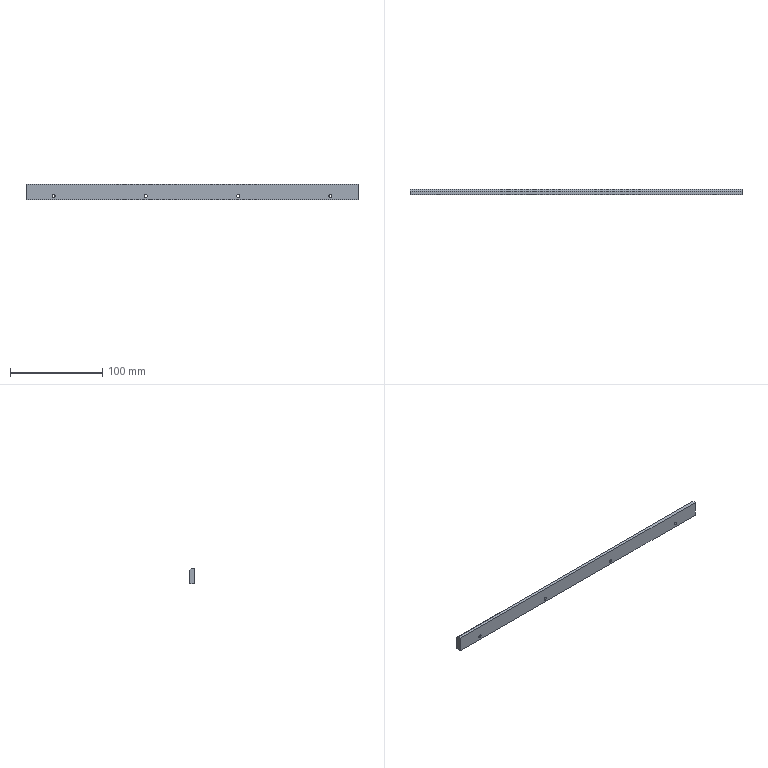Part | STEP file | PN_0029 | 1 solid | 15 faces | box 360 x 5.4 x 16.8 mm | volume 31743 mm3 | cylinder 8 | plane 7 | commonest cylinder face diameters 3.4 x8
STEP:
#1=CARTESIAN_POINT('',(0.,0.,0.));
#2=DIRECTION('',(0.,0.,1.));
#3=DIRECTION('',(1.,0.,0.));
#4=AXIS2_PLACEMENT_3D('',#1,#2,#3);
#5=CARTESIAN_POINT('',(-150.,0.,-2.7));
#6=VERTEX_POINT('',#5);
#7=CARTESIAN_POINT('',(-150.,5.4,-2.7));
#8=VERTEX_POINT('',#7);
#9=CARTESIAN_POINT('',(-150.,5.4,-2.7));
#10=DIRECTION('',(0.,1.,0.));
#11=VECTOR('',#10,1.);
#12=LINE('',#9,#11);
#13=CARTESIAN_POINT('',(-150.,5.4,-4.4));
#14=DIRECTION('',(0.,1.,0.));
#15=DIRECTION('',(0.,0.,1.));
#16=AXIS2_PLACEMENT_3D('',#13,#14,#15);
#17=CYLINDRICAL_SURFACE('',#16,1.7);
#18=CARTESIAN_POINT('',(6.283,0.));
#19=DIRECTION('',(0.,1.));
#20=VECTOR('',#19,1.);
#21=LINE('',#18,#20);
#22=(GEOMETRIC_REPRESENTATION_CONTEXT(2)PARAMETRIC_REPRESENTATION_CONTEXT()REPRESENTATION_CONTEXT('',''));
#23=DEFINITIONAL_REPRESENTATION('',(#21),#22);
#24=PCURVE('',#17,#23);
#25=CARTESIAN_POINT('',(-150.,5.4,-4.4));
#26=DIRECTION('',(0.,1.,0.));
#27=DIRECTION('',(0.,0.,1.));
#28=AXIS2_PLACEMENT_3D('',#25,#26,#27);
#29=CYLINDRICAL_SURFACE('',#28,1.7);
#30=CARTESIAN_POINT('',(0.,0.));
#31=DIRECTION('',(0.,1.));
#32=VECTOR('',#31,1.);
#33=LINE('',#30,#32);
#34=(GEOMETRIC_REPRESENTATION_CONTEXT(2)PARAMETRIC_REPRESENTATION_CONTEXT()REPRESENTATION_CONTEXT('',''));
#35=DEFINITIONAL_REPRESENTATION('',(#33),#34);
#36=PCURVE('',#29,#35);
#37=SURFACE_CURVE('',#12,(#24,#36),.PCURVE_S1.);
#38=EDGE_CURVE('',#6,#8,#37,.T.);
#39=ORIENTED_EDGE('',*,*,#38,.T.);
#40=CARTESIAN_POINT('',(-150.,5.4,-6.1));
#41=VERTEX_POINT('',#40);
#42=CARTESIAN_POINT('',(-150.,5.4,-4.4));
#43=DIRECTION('',(0.,1.,0.));
#44=DIRECTION('',(0.,0.,1.));
#45=AXIS2_PLACEMENT_3D('',#42,#43,#44);
#46=CIRCLE('',#45,1.7);
#47=CARTESIAN_POINT('',(0.,0.));
#48=DIRECTION('',(1.,0.));
#49=VECTOR('',#48,1.);
#50=LINE('',#47,#49);
#51=(GEOMETRIC_REPRESENTATION_CONTEXT(2)PARAMETRIC_REPRESENTATION_CONTEXT()REPRESENTATION_CONTEXT('',''));
#52=DEFINITIONAL_REPRESENTATION('',(#50),#51);
#53=PCURVE('',#17,#52);
#54=CARTESIAN_POINT('',(0.,5.4,0.));
#55=DIRECTION('',(0.,1.,0.));
#56=DIRECTION('',(0.,0.,1.));
#57=AXIS2_PLACEMENT_3D('',#54,#55,#56);
#58=PLANE('',#57);
#59=CARTESIAN_POINT('',(-4.4,-150.));
#60=DIRECTION('',(1.,0.));
#61=AXIS2_PLACEMENT_2D('',#59,#60);
#62=CIRCLE('',#61,1.7);
#63=(GEOMETRIC_REPRESENTATION_CONTEXT(2)PARAMETRIC_REPRESENTATION_CONTEXT()REPRESENTATION_CONTEXT('',''));
#64=DEFINITIONAL_REPRESENTATION('',(#62),#63);
#65=PCURVE('',#58,#64);
#66=SURFACE_CURVE('',#46,(#53,#65),.PCURVE_S1.);
#67=EDGE_CURVE('',#41,#8,#66,.T.);
#68=ORIENTED_EDGE('',*,*,#67,.F.);
#69=CARTESIAN_POINT('',(-150.,0.,-6.1));
#70=VERTEX_POINT('',#69);
#71=CARTESIAN_POINT('',(-150.,5.4,-6.1));
#72=DIRECTION('',(0.,1.,0.));
#73=VECTOR('',#72,1.);
#74=LINE('',#71,#73);
#75=CARTESIAN_POINT('',(3.142,0.));
#76=DIRECTION('',(0.,1.));
#77=VECTOR('',#76,1.);
#78=LINE('',#75,#77);
#79=(GEOMETRIC_REPRESENTATION_CONTEXT(2)PARAMETRIC_REPRESENTATION_CONTEXT()REPRESENTATION_CONTEXT('',''));
#80=DEFINITIONAL_REPRESENTATION('',(#78),#79);
#81=PCURVE('',#17,#80);
#82=CARTESIAN_POINT('',(3.142,0.));
#83=DIRECTION('',(0.,1.));
#84=VECTOR('',#83,1.);
#85=LINE('',#82,#84);
#86=(GEOMETRIC_REPRESENTATION_CONTEXT(2)PARAMETRIC_REPRESENTATION_CONTEXT()REPRESENTATION_CONTEXT('',''));
#87=DEFINITIONAL_REPRESENTATION('',(#85),#86);
#88=PCURVE('',#29,#87);
#89=SURFACE_CURVE('',#74,(#81,#88),.PCURVE_S1.);
#90=EDGE_CURVE('',#70,#41,#89,.T.);
#91=ORIENTED_EDGE('',*,*,#90,.F.);
#92=CARTESIAN_POINT('',(-150.,0.,-4.4));
#93=DIRECTION('',(0.,1.,0.));
#94=DIRECTION('',(0.,0.,1.));
#95=AXIS2_PLACEMENT_3D('',#92,#93,#94);
#96=CIRCLE('',#95,1.7);
#97=CARTESIAN_POINT('',(0.,-5.4));
#98=DIRECTION('',(1.,0.));
#99=VECTOR('',#98,1.);
#100=LINE('',#97,#99);
#101=(GEOMETRIC_REPRESENTATION_CONTEXT(2)PARAMETRIC_REPRESENTATION_CONTEXT()REPRESENTATION_CONTEXT('',''));
#102=DEFINITIONAL_REPRESENTATION('',(#100),#101);
#103=PCURVE('',#17,#102);
#104=CARTESIAN_POINT('',(0.,0.,0.));
#105=DIRECTION('',(0.,1.,0.));
#106=DIRECTION('',(0.,0.,1.));
#107=AXIS2_PLACEMENT_3D('',#104,#105,#106);
#108=PLANE('',#107);
#109=CARTESIAN_POINT('',(-4.4,-150.));
#110=DIRECTION('',(1.,0.));
#111=AXIS2_PLACEMENT_2D('',#109,#110);
#112=CIRCLE('',#111,1.7);
#113=(GEOMETRIC_REPRESENTATION_CONTEXT(2)PARAMETRIC_REPRESENTATION_CONTEXT()REPRESENTATION_CONTEXT('',''));
#114=DEFINITIONAL_REPRESENTATION('',(#112),#113);
#115=PCURVE('',#108,#114);
#116=SURFACE_CURVE('',#96,(#103,#115),.PCURVE_S1.);
#117=EDGE_CURVE('',#70,#6,#116,.T.);
#118=ORIENTED_EDGE('',*,*,#117,.T.);
#119=EDGE_LOOP('',(#39,#68,#91,#118));
#120=FACE_BOUND('',#119,.F.);
#121=ADVANCED_FACE('',(#120),#17,.F.);
#122=CARTESIAN_POINT('',(-50.,0.,-2.7));
#123=VERTEX_POINT('',#122);
#124=CARTESIAN_POINT('',(-50.,5.4,-2.7));
#125=VERTEX_POINT('',#124);
#126=CARTESIAN_POINT('',(-50.,5.4,-2.7));
#127=DIRECTION('',(0.,1.,0.));
#128=VECTOR('',#127,1.);
#129=LINE('',#126,#128);
#130=CARTESIAN_POINT('',(-50.,5.4,-4.4));
#131=DIRECTION('',(0.,1.,0.));
#132=DIRECTION('',(0.,0.,1.));
#133=AXIS2_PLACEMENT_3D('',#130,#131,#132);
#134=CYLINDRICAL_SURFACE('',#133,1.7);
#135=CARTESIAN_POINT('',(6.283,0.));
#136=DIRECTION('',(0.,1.));
#137=VECTOR('',#136,1.);
#138=LINE('',#135,#137);
#139=(GEOMETRIC_REPRESENTATION_CONTEXT(2)PARAMETRIC_REPRESENTATION_CONTEXT()REPRESENTATION_CONTEXT('',''));
#140=DEFINITIONAL_REPRESENTATION('',(#138),#139);
#141=PCURVE('',#134,#140);
#142=CARTESIAN_POINT('',(-50.,5.4,-4.4));
#143=DIRECTION('',(0.,1.,0.));
#144=DIRECTION('',(0.,0.,1.));
#145=AXIS2_PLACEMENT_3D('',#142,#143,#144);
#146=CYLINDRICAL_SURFACE('',#145,1.7);
#147=CARTESIAN_POINT('',(0.,0.));
#148=DIRECTION('',(0.,1.));
#149=VECTOR('',#148,1.);
#150=LINE('',#147,#149);
#151=(GEOMETRIC_REPRESENTATION_CONTEXT(2)PARAMETRIC_REPRESENTATION_CONTEXT()REPRESENTATION_CONTEXT('',''));
#152=DEFINITIONAL_REPRESENTATION('',(#150),#151);
#153=PCURVE('',#146,#152);
#154=SURFACE_CURVE('',#129,(#141,#153),.PCURVE_S1.);
#155=EDGE_CURVE('',#123,#125,#154,.T.);
#156=ORIENTED_EDGE('',*,*,#155,.T.);
#157=CARTESIAN_POINT('',(-50.,5.4,-6.1));
#158=VERTEX_POINT('',#157);
#159=CARTESIAN_POINT('',(-50.,5.4,-4.4));
#160=DIRECTION('',(0.,1.,0.));
#161=DIRECTION('',(0.,0.,1.));
#162=AXIS2_PLACEMENT_3D('',#159,#160,#161);
#163=CIRCLE('',#162,1.7);
#164=CARTESIAN_POINT('',(0.,0.));
#165=DIRECTION('',(1.,0.));
#166=VECTOR('',#165,1.);
#167=LINE('',#164,#166);
#168=(GEOMETRIC_REPRESENTATION_CONTEXT(2)PARAMETRIC_REPRESENTATION_CONTEXT()REPRESENTATION_CONTEXT('',''));
#169=DEFINITIONAL_REPRESENTATION('',(#167),#168);
#170=PCURVE('',#134,#169);
#171=CARTESIAN_POINT('',(-4.4,-50.));
#172=DIRECTION('',(1.,0.));
#173=AXIS2_PLACEMENT_2D('',#171,#172);
#174=CIRCLE('',#173,1.7);
#175=(GEOMETRIC_REPRESENTATION_CONTEXT(2)PARAMETRIC_REPRESENTATION_CONTEXT()REPRESENTATION_CONTEXT('',''));
#176=DEFINITIONAL_REPRESENTATION('',(#174),#175);
#177=PCURVE('',#58,#176);
#178=SURFACE_CURVE('',#163,(#170,#177),.PCURVE_S1.);
#179=EDGE_CURVE('',#158,#125,#178,.T.);
#180=ORIENTED_EDGE('',*,*,#179,.F.);
#181=CARTESIAN_POINT('',(-50.,0.,-6.1));
#182=VERTEX_POINT('',#181);
#183=CARTESIAN_POINT('',(-50.,5.4,-6.1));
#184=DIRECTION('',(0.,1.,0.));
#185=VECTOR('',#184,1.);
#186=LINE('',#183,#185);
#187=CARTESIAN_POINT('',(3.142,0.));
#188=DIRECTION('',(0.,1.));
#189=VECTOR('',#188,1.);
#190=LINE('',#187,#189);
#191=(GEOMETRIC_REPRESENTATION_CONTEXT(2)PARAMETRIC_REPRESENTATION_CONTEXT()REPRESENTATION_CONTEXT('',''));
#192=DEFINITIONAL_REPRESENTATION('',(#190),#191);
#193=PCURVE('',#134,#192);
#194=CARTESIAN_POINT('',(3.142,0.));
#195=DIRECTION('',(0.,1.));
#196=VECTOR('',#195,1.);
#197=LINE('',#194,#196);
#198=(GEOMETRIC_REPRESENTATION_CONTEXT(2)PARAMETRIC_REPRESENTATION_CONTEXT()REPRESENTATION_CONTEXT('',''));
#199=DEFINITIONAL_REPRESENTATION('',(#197),#198);
#200=PCURVE('',#146,#199);
#201=SURFACE_CURVE('',#186,(#193,#200),.PCURVE_S1.);
#202=EDGE_CURVE('',#182,#158,#201,.T.);
#203=ORIENTED_EDGE('',*,*,#202,.F.);
#204=CARTESIAN_POINT('',(-50.,0.,-4.4));
#205=DIRECTION('',(0.,1.,0.));
#206=DIRECTION('',(0.,0.,1.));
#207=AXIS2_PLACEMENT_3D('',#204,#205,#206);
#208=CIRCLE('',#207,1.7);
#209=CARTESIAN_POINT('',(0.,-5.4));
#210=DIRECTION('',(1.,0.));
#211=VECTOR('',#210,1.);
#212=LINE('',#209,#211);
#213=(GEOMETRIC_REPRESENTATION_CONTEXT(2)PARAMETRIC_REPRESENTATION_CONTEXT()REPRESENTATION_CONTEXT('',''));
#214=DEFINITIONAL_REPRESENTATION('',(#212),#213);
#215=PCURVE('',#134,#214);
#216=CARTESIAN_POINT('',(-4.4,-50.));
#217=DIRECTION('',(1.,0.));
#218=AXIS2_PLACEMENT_2D('',#216,#217);
#219=CIRCLE('',#218,1.7);
#220=(GEOMETRIC_REPRESENTATION_CONTEXT(2)PARAMETRIC_REPRESENTATION_CONTEXT()REPRESENTATION_CONTEXT('',''));
#221=DEFINITIONAL_REPRESENTATION('',(#219),#220);
#222=PCURVE('',#108,#221);
#223=SURFACE_CURVE('',#208,(#215,#222),.PCURVE_S1.);
#224=EDGE_CURVE('',#182,#123,#223,.T.);
#225=ORIENTED_EDGE('',*,*,#224,.T.);
#226=EDGE_LOOP('',(#156,#180,#203,#225));
#227=FACE_BOUND('',#226,.F.);
#228=ADVANCED_FACE('',(#227),#134,.F.);
#229=CARTESIAN_POINT('',(50.,0.,-2.7));
#230=VERTEX_POINT('',#229);
#231=CARTESIAN_POINT('',(50.,5.4,-2.7));
#232=VERTEX_POINT('',#231);
#233=CARTESIAN_POINT('',(50.,5.4,-2.7));
#234=DIRECTION('',(0.,1.,0.));
#235=VECTOR('',#234,1.);
#236=LINE('',#233,#235);
#237=CARTESIAN_POINT('',(50.,5.4,-4.4));
#238=DIRECTION('',(0.,1.,0.));
#239=DIRECTION('',(0.,0.,1.));
#240=AXIS2_PLACEMENT_3D('',#237,#238,#239);
#241=CYLINDRICAL_SURFACE('',#240,1.7);
#242=CARTESIAN_POINT('',(6.283,0.));
#243=DIRECTION('',(0.,1.));
#244=VECTOR('',#243,1.);
#245=LINE('',#242,#244);
#246=(GEOMETRIC_REPRESENTATION_CONTEXT(2)PARAMETRIC_REPRESENTATION_CONTEXT()REPRESENTATION_CONTEXT('',''));
#247=DEFINITIONAL_REPRESENTATION('',(#245),#246);
#248=PCURVE('',#241,#247);
#249=CARTESIAN_POINT('',(50.,5.4,-4.4));
#250=DIRECTION('',(0.,1.,0.));
#251=DIRECTION('',(0.,0.,1.));
#252=AXIS2_PLACEMENT_3D('',#249,#250,#251);
#253=CYLINDRICAL_SURFACE('',#252,1.7);
#254=CARTESIAN_POINT('',(0.,0.));
#255=DIRECTION('',(0.,1.));
#256=VECTOR('',#255,1.);
#257=LINE('',#254,#256);
#258=(GEOMETRIC_REPRESENTATION_CONTEXT(2)PARAMETRIC_REPRESENTATION_CONTEXT()REPRESENTATION_CONTEXT('',''));
#259=DEFINITIONAL_REPRESENTATION('',(#257),#258);
#260=PCURVE('',#253,#259);
#261=SURFACE_CURVE('',#236,(#248,#260),.PCURVE_S1.);
#262=EDGE_CURVE('',#230,#232,#261,.T.);
#263=ORIENTED_EDGE('',*,*,#262,.T.);
#264=CARTESIAN_POINT('',(50.,5.4,-6.1));
#265=VERTEX_POINT('',#264);
#266=CARTESIAN_POINT('',(50.,5.4,-4.4));
#267=DIRECTION('',(0.,1.,0.));
#268=DIRECTION('',(0.,0.,1.));
#269=AXIS2_PLACEMENT_3D('',#266,#267,#268);
#270=CIRCLE('',#269,1.7);
#271=CARTESIAN_POINT('',(0.,0.));
#272=DIRECTION('',(1.,0.));
#273=VECTOR('',#272,1.);
#274=LINE('',#271,#273);
#275=(GEOMETRIC_REPRESENTATION_CONTEXT(2)PARAMETRIC_REPRESENTATION_CONTEXT()REPRESENTATION_CONTEXT('',''));
#276=DEFINITIONAL_REPRESENTATION('',(#274),#275);
#277=PCURVE('',#241,#276);
#278=CARTESIAN_POINT('',(-4.4,50.));
#279=DIRECTION('',(1.,0.));
#280=AXIS2_PLACEMENT_2D('',#278,#279);
#281=CIRCLE('',#280,1.7);
#282=(GEOMETRIC_REPRESENTATION_CONTEXT(2)PARAMETRIC_REPRESENTATION_CONTEXT()REPRESENTATION_CONTEXT('',''));
#283=DEFINITIONAL_REPRESENTATION('',(#281),#282);
#284=PCURVE('',#58,#283);
#285=SURFACE_CURVE('',#270,(#277,#284),.PCURVE_S1.);
#286=EDGE_CURVE('',#265,#232,#285,.T.);
#287=ORIENTED_EDGE('',*,*,#286,.F.);
#288=CARTESIAN_POINT('',(50.,0.,-6.1));
#289=VERTEX_POINT('',#288);
#290=CARTESIAN_POINT('',(50.,5.4,-6.1));
#291=DIRECTION('',(0.,1.,0.));
#292=VECTOR('',#291,1.);
#293=LINE('',#290,#292);
#294=CARTESIAN_POINT('',(3.142,0.));
#295=DIRECTION('',(0.,1.));
#296=VECTOR('',#295,1.);
#297=LINE('',#294,#296);
#298=(GEOMETRIC_REPRESENTATION_CONTEXT(2)PARAMETRIC_REPRESENTATION_CONTEXT()REPRESENTATION_CONTEXT('',''));
#299=DEFINITIONAL_REPRESENTATION('',(#297),#298);
#300=PCURVE('',#241,#299);
#301=CARTESIAN_POINT('',(3.142,0.));
#302=DIRECTION('',(0.,1.));
#303=VECTOR('',#302,1.);
#304=LINE('',#301,#303);
#305=(GEOMETRIC_REPRESENTATION_CONTEXT(2)PARAMETRIC_REPRESENTATION_CONTEXT()REPRESENTATION_CONTEXT('',''));
#306=DEFINITIONAL_REPRESENTATION('',(#304),#305);
#307=PCURVE('',#253,#306);
#308=SURFACE_CURVE('',#293,(#300,#307),.PCURVE_S1.);
#309=EDGE_CURVE('',#289,#265,#308,.T.);
#310=ORIENTED_EDGE('',*,*,#309,.F.);
#311=CARTESIAN_POINT('',(50.,0.,-4.4));
#312=DIRECTION('',(0.,1.,0.));
#313=DIRECTION('',(0.,0.,1.));
#314=AXIS2_PLACEMENT_3D('',#311,#312,#313);
#315=CIRCLE('',#314,1.7);
#316=CARTESIAN_POINT('',(0.,-5.4));
#317=DIRECTION('',(1.,0.));
#318=VECTOR('',#317,1.);
#319=LINE('',#316,#318);
#320=(GEOMETRIC_REPRESENTATION_CONTEXT(2)PARAMETRIC_REPRESENTATION_CONTEXT()REPRESENTATION_CONTEXT('',''));
#321=DEFINITIONAL_REPRESENTATION('',(#319),#320);
#322=PCURVE('',#241,#321);
#323=CARTESIAN_POINT('',(-4.4,50.));
#324=DIRECTION('',(1.,0.));
#325=AXIS2_PLACEMENT_2D('',#323,#324);
#326=CIRCLE('',#325,1.7);
#327=(GEOMETRIC_REPRESENTATION_CONTEXT(2)PARAMETRIC_REPRESENTATION_CONTEXT()REPRESENTATION_CONTEXT('',''));
#328=DEFINITIONAL_REPRESENTATION('',(#326),#327);
#329=PCURVE('',#108,#328);
#330=SURFACE_CURVE('',#315,(#322,#329),.PCURVE_S1.);
#331=EDGE_CURVE('',#289,#230,#330,.T.);
#332=ORIENTED_EDGE('',*,*,#331,.T.);
#333=EDGE_LOOP('',(#263,#287,#310,#332));
#334=FACE_BOUND('',#333,.F.);
#335=ADVANCED_FACE('',(#334),#241,.F.);
#336=CARTESIAN_POINT('',(150.,0.,-2.7));
#337=VERTEX_POINT('',#336);
#338=CARTESIAN_POINT('',(150.,5.4,-2.7));
#339=VERTEX_POINT('',#338);
#340=CARTESIAN_POINT('',(150.,5.4,-2.7));
#341=DIRECTION('',(0.,1.,0.));
#342=VECTOR('',#341,1.);
#343=LINE('',#340,#342);
#344=CARTESIAN_POINT('',(150.,5.4,-4.4));
#345=DIRECTION('',(0.,1.,0.));
#346=DIRECTION('',(0.,0.,1.));
#347=AXIS2_PLACEMENT_3D('',#344,#345,#346);
#348=CYLINDRICAL_SURFACE('',#347,1.7);
#349=CARTESIAN_POINT('',(6.283,0.));
#350=DIRECTION('',(0.,1.));
#351=VECTOR('',#350,1.);
#352=LINE('',#349,#351);
#353=(GEOMETRIC_REPRESENTATION_CONTEXT(2)PARAMETRIC_REPRESENTATION_CONTEXT()REPRESENTATION_CONTEXT('',''));
#354=DEFINITIONAL_REPRESENTATION('',(#352),#353);
#355=PCURVE('',#348,#354);
#356=CARTESIAN_POINT('',(150.,5.4,-4.4));
#357=DIRECTION('',(0.,1.,0.));
#358=DIRECTION('',(0.,0.,1.));
#359=AXIS2_PLACEMENT_3D('',#356,#357,#358);
#360=CYLINDRICAL_SURFACE('',#359,1.7);
#361=CARTESIAN_POINT('',(0.,0.));
#362=DIRECTION('',(0.,1.));
#363=VECTOR('',#362,1.);
#364=LINE('',#361,#363);
#365=(GEOMETRIC_REPRESENTATION_CONTEXT(2)PARAMETRIC_REPRESENTATION_CONTEXT()REPRESENTATION_CONTEXT('',''));
#366=DEFINITIONAL_REPRESENTATION('',(#364),#365);
#367=PCURVE('',#360,#366);
#368=SURFACE_CURVE('',#343,(#355,#367),.PCURVE_S1.);
#369=EDGE_CURVE('',#337,#339,#368,.T.);
#370=ORIENTED_EDGE('',*,*,#369,.T.);
#371=CARTESIAN_POINT('',(150.,5.4,-6.1));
#372=VERTEX_POINT('',#371);
#373=CARTESIAN_POINT('',(150.,5.4,-4.4));
#374=DIRECTION('',(0.,1.,0.));
#375=DIRECTION('',(0.,0.,1.));
#376=AXIS2_PLACEMENT_3D('',#373,#374,#375);
#377=CIRCLE('',#376,1.7);
#378=CARTESIAN_POINT('',(0.,0.));
#379=DIRECTION('',(1.,0.));
#380=VECTOR('',#379,1.);
#381=LINE('',#378,#380);
#382=(GEOMETRIC_REPRESENTATION_CONTEXT(2)PARAMETRIC_REPRESENTATION_CONTEXT()REPRESENTATION_CONTEXT('',''));
#383=DEFINITIONAL_REPRESENTATION('',(#381),#382);
#384=PCURVE('',#348,#383);
#385=CARTESIAN_POINT('',(-4.4,150.));
#386=DIRECTION('',(1.,0.));
#387=AXIS2_PLACEMENT_2D('',#385,#386);
#388=CIRCLE('',#387,1.7);
#389=(GEOMETRIC_REPRESENTATION_CONTEXT(2)PARAMETRIC_REPRESENTATION_CONTEXT()REPRESENTATION_CONTEXT('',''));
#390=DEFINITIONAL_REPRESENTATION('',(#388),#389);
#391=PCURVE('',#58,#390);
#392=SURFACE_CURVE('',#377,(#384,#391),.PCURVE_S1.);
#393=EDGE_CURVE('',#372,#339,#392,.T.);
#394=ORIENTED_EDGE('',*,*,#393,.F.);
#395=CARTESIAN_POINT('',(150.,0.,-6.1));
#396=VERTEX_POINT('',#395);
#397=CARTESIAN_POINT('',(150.,5.4,-6.1));
#398=DIRECTION('',(0.,1.,0.));
#399=VECTOR('',#398,1.);
#400=LINE('',#397,#399);
#401=CARTESIAN_POINT('',(3.142,0.));
#402=DIRECTION('',(0.,1.));
#403=VECTOR('',#402,1.);
#404=LINE('',#401,#403);
#405=(GEOMETRIC_REPRESENTATION_CONTEXT(2)PARAMETRIC_REPRESENTATION_CONTEXT()REPRESENTATION_CONTEXT('',''));
#406=DEFINITIONAL_REPRESENTATION('',(#404),#405);
#407=PCURVE('',#348,#406);
#408=CARTESIAN_POINT('',(3.142,0.));
#409=DIRECTION('',(0.,1.));
#410=VECTOR('',#409,1.);
#411=LINE('',#408,#410);
#412=(GEOMETRIC_REPRESENTATION_CONTEXT(2)PARAMETRIC_REPRESENTATION_CONTEXT()REPRESENTATION_CONTEXT('',''));
#413=DEFINITIONAL_REPRESENTATION('',(#411),#412);
#414=PCURVE('',#360,#413);
#415=SURFACE_CURVE('',#400,(#407,#414),.PCURVE_S1.);
#416=EDGE_CURVE('',#396,#372,#415,.T.);
#417=ORIENTED_EDGE('',*,*,#416,.F.);
#418=CARTESIAN_POINT('',(150.,0.,-4.4));
#419=DIRECTION('',(0.,1.,0.));
#420=DIRECTION('',(0.,0.,1.));
#421=AXIS2_PLACEMENT_3D('',#418,#419,#420);
#422=CIRCLE('',#421,1.7);
#423=CARTESIAN_POINT('',(0.,-5.4));
#424=DIRECTION('',(1.,0.));
#425=VECTOR('',#424,1.);
#426=LINE('',#423,#425);
#427=(GEOMETRIC_REPRESENTATION_CONTEXT(2)PARAMETRIC_REPRESENTATION_CONTEXT()REPRESENTATION_CONTEXT('',''));
#428=DEFINITIONAL_REPRESENTATION('',(#426),#427);
#429=PCURVE('',#348,#428);
#430=CARTESIAN_POINT('',(-4.4,150.));
#431=DIRECTION('',(1.,0.));
#432=AXIS2_PLACEMENT_2D('',#430,#431);
#433=CIRCLE('',#432,1.7);
#434=(GEOMETRIC_REPRESENTATION_CONTEXT(2)PARAMETRIC_REPRESENTATION_CONTEXT()REPRESENTATION_CONTEXT('',''));
#435=DEFINITIONAL_REPRESENTATION('',(#433),#434);
#436=PCURVE('',#108,#435);
#437=SURFACE_CURVE('',#422,(#429,#436),.PCURVE_S1.);
#438=EDGE_CURVE('',#396,#337,#437,.T.);
#439=ORIENTED_EDGE('',*,*,#438,.T.);
#440=EDGE_LOOP('',(#370,#394,#417,#439));
#441=FACE_BOUND('',#440,.F.);
#442=ADVANCED_FACE('',(#441),#348,.F.);
#443=CARTESIAN_POINT('',(180.,5.4,6.4));
#444=VERTEX_POINT('',#443);
#445=CARTESIAN_POINT('',(180.,5.4,-8.4));
#446=VERTEX_POINT('',#445);
#447=CARTESIAN_POINT('',(180.,5.4,-8.4));
#448=DIRECTION('',(0.,0.,-1.));
#449=VECTOR('',#448,1.);
#450=LINE('',#447,#449);
#451=CARTESIAN_POINT('',(180.,5.4,-8.4));
#452=DIRECTION('',(-1.,0.,0.));
#453=DIRECTION('',(0.,0.,1.));
#454=AXIS2_PLACEMENT_3D('',#451,#452,#453);
#455=PLANE('',#454);
#456=CARTESIAN_POINT('',(0.,0.));
#457=DIRECTION('',(-1.,0.));
#458=VECTOR('',#457,1.);
#459=LINE('',#456,#458);
#460=(GEOMETRIC_REPRESENTATION_CONTEXT(2)PARAMETRIC_REPRESENTATION_CONTEXT()REPRESENTATION_CONTEXT('',''));
#461=DEFINITIONAL_REPRESENTATION('',(#459),#460);
#462=PCURVE('',#455,#461);
#463=CARTESIAN_POINT('',(-8.4,180.));
#464=DIRECTION('',(-1.,0.));
#465=VECTOR('',#464,1.);
#466=LINE('',#463,#465);
#467=(GEOMETRIC_REPRESENTATION_CONTEXT(2)PARAMETRIC_REPRESENTATION_CONTEXT()REPRESENTATION_CONTEXT('',''));
#468=DEFINITIONAL_REPRESENTATION('',(#466),#467);
#469=PCURVE('',#58,#468);
#470=SURFACE_CURVE('',#450,(#462,#469),.PCURVE_S1.);
#471=EDGE_CURVE('',#444,#446,#470,.T.);
#472=ORIENTED_EDGE('',*,*,#471,.F.);
#473=CARTESIAN_POINT('',(180.,3.4,8.4));
#474=VERTEX_POINT('',#473);
#475=CARTESIAN_POINT('',(180.,3.4,8.4));
#476=DIRECTION('',(0.,-0.7071,0.7071));
#477=VECTOR('',#476,1.);
#478=LINE('',#475,#477);
#479=CARTESIAN_POINT('',(16.8,-2.));
#480=DIRECTION('',(0.7071,-0.7071));
#481=VECTOR('',#480,1.);
#482=LINE('',#479,#481);
#483=(GEOMETRIC_REPRESENTATION_CONTEXT(2)PARAMETRIC_REPRESENTATION_CONTEXT()REPRESENTATION_CONTEXT('',''));
#484=DEFINITIONAL_REPRESENTATION('',(#482),#483);
#485=PCURVE('',#455,#484);
#486=CARTESIAN_POINT('',(180.,3.4,8.4));
#487=DIRECTION('',(0.,-0.7071,-0.7071));
#488=DIRECTION('',(0.,0.7071,-0.7071));
#489=AXIS2_PLACEMENT_3D('',#486,#487,#488);
#490=PLANE('',#489);
#491=CARTESIAN_POINT('',(0.,0.));
#492=DIRECTION('',(-1.,0.));
#493=VECTOR('',#492,1.);
#494=LINE('',#491,#493);
#495=(GEOMETRIC_REPRESENTATION_CONTEXT(2)PARAMETRIC_REPRESENTATION_CONTEXT()REPRESENTATION_CONTEXT('',''));
#496=DEFINITIONAL_REPRESENTATION('',(#494),#495);
#497=PCURVE('',#490,#496);
#498=SURFACE_CURVE('',#478,(#485,#497),.PCURVE_S1.);
#499=EDGE_CURVE('',#444,#474,#498,.T.);
#500=ORIENTED_EDGE('',*,*,#499,.T.);
#501=CARTESIAN_POINT('',(180.,0.,8.4));
#502=VERTEX_POINT('',#501);
#503=CARTESIAN_POINT('',(180.,5.4,8.4));
#504=DIRECTION('',(0.,-1.,0.));
#505=VECTOR('',#504,1.);
#506=LINE('',#503,#505);
#507=CARTESIAN_POINT('',(16.8,0.));
#508=DIRECTION('',(0.,-1.));
#509=VECTOR('',#508,1.);
#510=LINE('',#507,#509);
#511=(GEOMETRIC_REPRESENTATION_CONTEXT(2)PARAMETRIC_REPRESENTATION_CONTEXT()REPRESENTATION_CONTEXT('',''));
#512=DEFINITIONAL_REPRESENTATION('',(#510),#511);
#513=PCURVE('',#455,#512);
#514=CARTESIAN_POINT('',(-180.,5.4,8.4));
#515=DIRECTION('',(0.,0.,-1.));
#516=DIRECTION('',(-1.,0.,0.));
#517=AXIS2_PLACEMENT_3D('',#514,#515,#516);
#518=PLANE('',#517);
#519=CARTESIAN_POINT('',(-360.,0.));
#520=DIRECTION('',(0.,-1.));
#521=VECTOR('',#520,1.);
#522=LINE('',#519,#521);
#523=(GEOMETRIC_REPRESENTATION_CONTEXT(2)PARAMETRIC_REPRESENTATION_CONTEXT()REPRESENTATION_CONTEXT('',''));
#524=DEFINITIONAL_REPRESENTATION('',(#522),#523);
#525=PCURVE('',#518,#524);
#526=SURFACE_CURVE('',#506,(#513,#525),.PCURVE_S1.);
#527=EDGE_CURVE('',#474,#502,#526,.T.);
#528=ORIENTED_EDGE('',*,*,#527,.T.);
#529=CARTESIAN_POINT('',(180.,0.,-8.4));
#530=VERTEX_POINT('',#529);
#531=CARTESIAN_POINT('',(180.,0.,-8.4));
#532=DIRECTION('',(0.,0.,-1.));
#533=VECTOR('',#532,1.);
#534=LINE('',#531,#533);
#535=CARTESIAN_POINT('',(0.,-5.4));
#536=DIRECTION('',(-1.,0.));
#537=VECTOR('',#536,1.);
#538=LINE('',#535,#537);
#539=(GEOMETRIC_REPRESENTATION_CONTEXT(2)PARAMETRIC_REPRESENTATION_CONTEXT()REPRESENTATION_CONTEXT('',''));
#540=DEFINITIONAL_REPRESENTATION('',(#538),#539);
#541=PCURVE('',#455,#540);
#542=CARTESIAN_POINT('',(-8.4,180.));
#543=DIRECTION('',(-1.,0.));
#544=VECTOR('',#543,1.);
#545=LINE('',#542,#544);
#546=(GEOMETRIC_REPRESENTATION_CONTEXT(2)PARAMETRIC_REPRESENTATION_CONTEXT()REPRESENTATION_CONTEXT('',''));
#547=DEFINITIONAL_REPRESENTATION('',(#545),#546);
#548=PCURVE('',#108,#547);
#549=SURFACE_CURVE('',#534,(#541,#548),.PCURVE_S1.);
#550=EDGE_CURVE('',#502,#530,#549,.T.);
#551=ORIENTED_EDGE('',*,*,#550,.T.);
#552=CARTESIAN_POINT('',(180.,5.4,-8.4));
#553=DIRECTION('',(0.,-1.,0.));
#554=VECTOR('',#553,1.);
#555=LINE('',#552,#554);
#556=CARTESIAN_POINT('',(0.,0.));
#557=DIRECTION('',(0.,-1.));
#558=VECTOR('',#557,1.);
#559=LINE('',#556,#558);
#560=(GEOMETRIC_REPRESENTATION_CONTEXT(2)PARAMETRIC_REPRESENTATION_CONTEXT()REPRESENTATION_CONTEXT('',''));
#561=DEFINITIONAL_REPRESENTATION('',(#559),#560);
#562=PCURVE('',#455,#561);
#563=CARTESIAN_POINT('',(-180.,5.4,-8.4));
#564=DIRECTION('',(0.,0.,1.));
#565=DIRECTION('',(1.,0.,0.));
#566=AXIS2_PLACEMENT_3D('',#563,#564,#565);
#567=PLANE('',#566);
#568=CARTESIAN_POINT('',(360.,0.));
#569=DIRECTION('',(0.,-1.));
#570=VECTOR('',#569,1.);
#571=LINE('',#568,#570);
#572=(GEOMETRIC_REPRESENTATION_CONTEXT(2)PARAMETRIC_REPRESENTATION_CONTEXT()REPRESENTATION_CONTEXT('',''));
#573=DEFINITIONAL_REPRESENTATION('',(#571),#572);
#574=PCURVE('',#567,#573);
#575=SURFACE_CURVE('',#555,(#562,#574),.PCURVE_S1.);
#576=EDGE_CURVE('',#446,#530,#575,.T.);
#577=ORIENTED_EDGE('',*,*,#576,.F.);
#578=EDGE_LOOP('',(#472,#500,#528,#551,#577));
#579=FACE_BOUND('',#578,.T.);
#580=ADVANCED_FACE('',(#579),#455,.F.);
#581=CARTESIAN_POINT('',(-180.,0.,-8.4));
#582=VERTEX_POINT('',#581);
#583=CARTESIAN_POINT('',(-180.,0.,-8.4));
#584=DIRECTION('',(-1.,0.,0.));
#585=VECTOR('',#584,1.);
#586=LINE('',#583,#585);
#587=CARTESIAN_POINT('',(0.,-5.4));
#588=DIRECTION('',(-1.,0.));
#589=VECTOR('',#588,1.);
#590=LINE('',#587,#589);
#591=(GEOMETRIC_REPRESENTATION_CONTEXT(2)PARAMETRIC_REPRESENTATION_CONTEXT()REPRESENTATION_CONTEXT('',''));
#592=DEFINITIONAL_REPRESENTATION('',(#590),#591);
#593=PCURVE('',#567,#592);
#594=CARTESIAN_POINT('',(-8.4,-180.));
#595=DIRECTION('',(0.,-1.));
#596=VECTOR('',#595,1.);
#597=LINE('',#594,#596);
#598=(GEOMETRIC_REPRESENTATION_CONTEXT(2)PARAMETRIC_REPRESENTATION_CONTEXT()REPRESENTATION_CONTEXT('',''));
#599=DEFINITIONAL_REPRESENTATION('',(#597),#598);
#600=PCURVE('',#108,#599);
#601=SURFACE_CURVE('',#586,(#593,#600),.PCURVE_S1.);
#602=EDGE_CURVE('',#530,#582,#601,.T.);
#603=ORIENTED_EDGE('',*,*,#602,.T.);
#604=CARTESIAN_POINT('',(-180.,5.4,-8.4));
#605=VERTEX_POINT('',#604);
#606=CARTESIAN_POINT('',(-180.,5.4,-8.4));
#607=DIRECTION('',(0.,-1.,0.));
#608=VECTOR('',#607,1.);
#609=LINE('',#606,#608);
#610=CARTESIAN_POINT('',(0.,0.));
#611=DIRECTION('',(0.,-1.));
#612=VECTOR('',#611,1.);
#613=LINE('',#610,#612);
#614=(GEOMETRIC_REPRESENTATION_CONTEXT(2)PARAMETRIC_REPRESENTATION_CONTEXT()REPRESENTATION_CONTEXT('',''));
#615=DEFINITIONAL_REPRESENTATION('',(#613),#614);
#616=PCURVE('',#567,#615);
#617=CARTESIAN_POINT('',(-180.,5.4,-8.4));
#618=DIRECTION('',(1.,0.,0.));
#619=DIRECTION('',(0.,0.,-1.));
#620=AXIS2_PLACEMENT_3D('',#617,#618,#619);
#621=PLANE('',#620);
#622=CARTESIAN_POINT('',(0.,0.));
#623=DIRECTION('',(0.,-1.));
#624=VECTOR('',#623,1.);
#625=LINE('',#622,#624);
#626=(GEOMETRIC_REPRESENTATION_CONTEXT(2)PARAMETRIC_REPRESENTATION_CONTEXT()REPRESENTATION_CONTEXT('',''));
#627=DEFINITIONAL_REPRESENTATION('',(#625),#626);
#628=PCURVE('',#621,#627);
#629=SURFACE_CURVE('',#609,(#616,#628),.PCURVE_S1.);
#630=EDGE_CURVE('',#605,#582,#629,.T.);
#631=ORIENTED_EDGE('',*,*,#630,.F.);
#632=CARTESIAN_POINT('',(-180.,5.4,-8.4));
#633=DIRECTION('',(-1.,0.,0.));
#634=VECTOR('',#633,1.);
#635=LINE('',#632,#634);
#636=CARTESIAN_POINT('',(0.,0.));
#637=DIRECTION('',(-1.,0.));
#638=VECTOR('',#637,1.);
#639=LINE('',#636,#638);
#640=(GEOMETRIC_REPRESENTATION_CONTEXT(2)PARAMETRIC_REPRESENTATION_CONTEXT()REPRESENTATION_CONTEXT('',''));
#641=DEFINITIONAL_REPRESENTATION('',(#639),#640);
#642=PCURVE('',#567,#641);
#643=CARTESIAN_POINT('',(-8.4,-180.));
#644=DIRECTION('',(0.,-1.));
#645=VECTOR('',#644,1.);
#646=LINE('',#643,#645);
#647=(GEOMETRIC_REPRESENTATION_CONTEXT(2)PARAMETRIC_REPRESENTATION_CONTEXT()REPRESENTATION_CONTEXT('',''));
#648=DEFINITIONAL_REPRESENTATION('',(#646),#647);
#649=PCURVE('',#58,#648);
#650=SURFACE_CURVE('',#635,(#642,#649),.PCURVE_S1.);
#651=EDGE_CURVE('',#446,#605,#650,.T.);
#652=ORIENTED_EDGE('',*,*,#651,.F.);
#653=ORIENTED_EDGE('',*,*,#576,.T.);
#654=EDGE_LOOP('',(#603,#631,#652,#653));
#655=FACE_BOUND('',#654,.T.);
#656=ADVANCED_FACE('',(#655),#567,.F.);
#657=CARTESIAN_POINT('',(-180.,3.4,8.4));
#658=VERTEX_POINT('',#657);
#659=CARTESIAN_POINT('',(-180.,0.,8.4));
#660=VERTEX_POINT('',#659);
#661=CARTESIAN_POINT('',(-180.,5.4,8.4));
#662=DIRECTION('',(0.,-1.,0.));
#663=VECTOR('',#662,1.);
#664=LINE('',#661,#663);
#665=CARTESIAN_POINT('',(-16.8,0.));
#666=DIRECTION('',(0.,-1.));
#667=VECTOR('',#666,1.);
#668=LINE('',#665,#667);
#669=(GEOMETRIC_REPRESENTATION_CONTEXT(2)PARAMETRIC_REPRESENTATION_CONTEXT()REPRESENTATION_CONTEXT('',''));
#670=DEFINITIONAL_REPRESENTATION('',(#668),#669);
#671=PCURVE('',#621,#670);
#672=CARTESIAN_POINT('',(0.,0.));
#673=DIRECTION('',(0.,-1.));
#674=VECTOR('',#673,1.);
#675=LINE('',#672,#674);
#676=(GEOMETRIC_REPRESENTATION_CONTEXT(2)PARAMETRIC_REPRESENTATION_CONTEXT()REPRESENTATION_CONTEXT('',''));
#677=DEFINITIONAL_REPRESENTATION('',(#675),#676);
#678=PCURVE('',#518,#677);
#679=SURFACE_CURVE('',#664,(#671,#678),.PCURVE_S1.);
#680=EDGE_CURVE('',#658,#660,#679,.T.);
#681=ORIENTED_EDGE('',*,*,#680,.F.);
#682=CARTESIAN_POINT('',(-180.,5.4,6.4));
#683=VERTEX_POINT('',#682);
#684=CARTESIAN_POINT('',(-180.,3.4,8.4));
#685=DIRECTION('',(0.,-0.7071,0.7071));
#686=VECTOR('',#685,1.);
#687=LINE('',#684,#686);
#688=CARTESIAN_POINT('',(-16.8,-2.));
#689=DIRECTION('',(-0.7071,-0.7071));
#690=VECTOR('',#689,1.);
#691=LINE('',#688,#690);
#692=(GEOMETRIC_REPRESENTATION_CONTEXT(2)PARAMETRIC_REPRESENTATION_CONTEXT()REPRESENTATION_CONTEXT('',''));
#693=DEFINITIONAL_REPRESENTATION('',(#691),#692);
#694=PCURVE('',#621,#693);
#695=CARTESIAN_POINT('',(0.,-360.));
#696=DIRECTION('',(-1.,0.));
#697=VECTOR('',#696,1.);
#698=LINE('',#695,#697);
#699=(GEOMETRIC_REPRESENTATION_CONTEXT(2)PARAMETRIC_REPRESENTATION_CONTEXT()REPRESENTATION_CONTEXT('',''));
#700=DEFINITIONAL_REPRESENTATION('',(#698),#699);
#701=PCURVE('',#490,#700);
#702=SURFACE_CURVE('',#687,(#694,#701),.PCURVE_S1.);
#703=EDGE_CURVE('',#683,#658,#702,.T.);
#704=ORIENTED_EDGE('',*,*,#703,.F.);
#705=CARTESIAN_POINT('',(-180.,5.4,-8.4));
#706=DIRECTION('',(0.,0.,1.));
#707=VECTOR('',#706,1.);
#708=LINE('',#705,#707);
#709=CARTESIAN_POINT('',(0.,0.));
#710=DIRECTION('',(-1.,0.));
#711=VECTOR('',#710,1.);
#712=LINE('',#709,#711);
#713=(GEOMETRIC_REPRESENTATION_CONTEXT(2)PARAMETRIC_REPRESENTATION_CONTEXT()REPRESENTATION_CONTEXT('',''));
#714=DEFINITIONAL_REPRESENTATION('',(#712),#713);
#715=PCURVE('',#621,#714);
#716=CARTESIAN_POINT('',(-8.4,-180.));
#717=DIRECTION('',(1.,0.));
#718=VECTOR('',#717,1.);
#719=LINE('',#716,#718);
#720=(GEOMETRIC_REPRESENTATION_CONTEXT(2)PARAMETRIC_REPRESENTATION_CONTEXT()REPRESENTATION_CONTEXT('',''));
#721=DEFINITIONAL_REPRESENTATION('',(#719),#720);
#722=PCURVE('',#58,#721);
#723=SURFACE_CURVE('',#708,(#715,#722),.PCURVE_S1.);
#724=EDGE_CURVE('',#605,#683,#723,.T.);
#725=ORIENTED_EDGE('',*,*,#724,.F.);
#726=ORIENTED_EDGE('',*,*,#630,.T.);
#727=CARTESIAN_POINT('',(-180.,0.,-8.4));
#728=DIRECTION('',(0.,0.,1.));
#729=VECTOR('',#728,1.);
#730=LINE('',#727,#729);
#731=CARTESIAN_POINT('',(0.,-5.4));
#732=DIRECTION('',(-1.,0.));
#733=VECTOR('',#732,1.);
#734=LINE('',#731,#733);
#735=(GEOMETRIC_REPRESENTATION_CONTEXT(2)PARAMETRIC_REPRESENTATION_CONTEXT()REPRESENTATION_CONTEXT('',''));
#736=DEFINITIONAL_REPRESENTATION('',(#734),#735);
#737=PCURVE('',#621,#736);
#738=CARTESIAN_POINT('',(-8.4,-180.));
#739=DIRECTION('',(1.,0.));
#740=VECTOR('',#739,1.);
#741=LINE('',#738,#740);
#742=(GEOMETRIC_REPRESENTATION_CONTEXT(2)PARAMETRIC_REPRESENTATION_CONTEXT()REPRESENTATION_CONTEXT('',''));
#743=DEFINITIONAL_REPRESENTATION('',(#741),#742);
#744=PCURVE('',#108,#743);
#745=SURFACE_CURVE('',#730,(#737,#744),.PCURVE_S1.);
#746=EDGE_CURVE('',#582,#660,#745,.T.);
#747=ORIENTED_EDGE('',*,*,#746,.T.);
#748=EDGE_LOOP('',(#681,#704,#725,#726,#747));
#749=FACE_BOUND('',#748,.T.);
#750=ADVANCED_FACE('',(#749),#621,.F.);
#751=ORIENTED_EDGE('',*,*,#527,.F.);
#752=CARTESIAN_POINT('',(180.,3.4,8.4));
#753=DIRECTION('',(-1.,0.,0.));
#754=VECTOR('',#753,1.);
#755=LINE('',#752,#754);
#756=CARTESIAN_POINT('',(-360.,-2.));
#757=DIRECTION('',(1.,0.));
#758=VECTOR('',#757,1.);
#759=LINE('',#756,#758);
#760=(GEOMETRIC_REPRESENTATION_CONTEXT(2)PARAMETRIC_REPRESENTATION_CONTEXT()REPRESENTATION_CONTEXT('',''));
#761=DEFINITIONAL_REPRESENTATION('',(#759),#760);
#762=PCURVE('',#518,#761);
#763=CARTESIAN_POINT('',(0.,0.));
#764=DIRECTION('',(0.,-1.));
#765=VECTOR('',#764,1.);
#766=LINE('',#763,#765);
#767=(GEOMETRIC_REPRESENTATION_CONTEXT(2)PARAMETRIC_REPRESENTATION_CONTEXT()REPRESENTATION_CONTEXT('',''));
#768=DEFINITIONAL_REPRESENTATION('',(#766),#767);
#769=PCURVE('',#490,#768);
#770=SURFACE_CURVE('',#755,(#762,#769),.PCURVE_S1.);
#771=EDGE_CURVE('',#474,#658,#770,.T.);
#772=ORIENTED_EDGE('',*,*,#771,.T.);
#773=ORIENTED_EDGE('',*,*,#680,.T.);
#774=CARTESIAN_POINT('',(-180.,0.,8.4));
#775=DIRECTION('',(1.,0.,0.));
#776=VECTOR('',#775,1.);
#777=LINE('',#774,#776);
#778=CARTESIAN_POINT('',(0.,-5.4));
#779=DIRECTION('',(-1.,0.));
#780=VECTOR('',#779,1.);
#781=LINE('',#778,#780);
#782=(GEOMETRIC_REPRESENTATION_CONTEXT(2)PARAMETRIC_REPRESENTATION_CONTEXT()REPRESENTATION_CONTEXT('',''));
#783=DEFINITIONAL_REPRESENTATION('',(#781),#782);
#784=PCURVE('',#518,#783);
#785=CARTESIAN_POINT('',(8.4,-180.));
#786=DIRECTION('',(0.,1.));
#787=VECTOR('',#786,1.);
#788=LINE('',#785,#787);
#789=(GEOMETRIC_REPRESENTATION_CONTEXT(2)PARAMETRIC_REPRESENTATION_CONTEXT()REPRESENTATION_CONTEXT('',''));
#790=DEFINITIONAL_REPRESENTATION('',(#788),#789);
#791=PCURVE('',#108,#790);
#792=SURFACE_CURVE('',#777,(#784,#791),.PCURVE_S1.);
#793=EDGE_CURVE('',#660,#502,#792,.T.);
#794=ORIENTED_EDGE('',*,*,#793,.T.);
#795=EDGE_LOOP('',(#751,#772,#773,#794));
#796=FACE_BOUND('',#795,.T.);
#797=ADVANCED_FACE('',(#796),#518,.F.);
#798=CARTESIAN_POINT('',(-150.,5.4,-4.4));
#799=DIRECTION('',(0.,1.,0.));
#800=DIRECTION('',(0.,0.,1.));
#801=AXIS2_PLACEMENT_3D('',#798,#799,#800);
#802=CIRCLE('',#801,1.7);
#803=CARTESIAN_POINT('',(-4.4,-150.));
#804=DIRECTION('',(1.,0.));
#805=AXIS2_PLACEMENT_2D('',#803,#804);
#806=CIRCLE('',#805,1.7);
#807=(GEOMETRIC_REPRESENTATION_CONTEXT(2)PARAMETRIC_REPRESENTATION_CONTEXT()REPRESENTATION_CONTEXT('',''));
#808=DEFINITIONAL_REPRESENTATION('',(#806),#807);
#809=PCURVE('',#58,#808);
#810=CARTESIAN_POINT('',(0.,0.));
#811=DIRECTION('',(1.,0.));
#812=VECTOR('',#811,1.);
#813=LINE('',#810,#812);
#814=(GEOMETRIC_REPRESENTATION_CONTEXT(2)PARAMETRIC_REPRESENTATION_CONTEXT()REPRESENTATION_CONTEXT('',''));
#815=DEFINITIONAL_REPRESENTATION('',(#813),#814);
#816=PCURVE('',#29,#815);
#817=SURFACE_CURVE('',#802,(#809,#816),.PCURVE_S1.);
#818=EDGE_CURVE('',#8,#41,#817,.T.);
#819=ORIENTED_EDGE('',*,*,#818,.F.);
#820=ORIENTED_EDGE('',*,*,#67,.F.);
#821=EDGE_LOOP('',(#819,#820));
#822=FACE_BOUND('',#821,.T.);
#823=CARTESIAN_POINT('',(-50.,5.4,-4.4));
#824=DIRECTION('',(0.,1.,0.));
#825=DIRECTION('',(0.,0.,1.));
#826=AXIS2_PLACEMENT_3D('',#823,#824,#825);
#827=CIRCLE('',#826,1.7);
#828=CARTESIAN_POINT('',(-4.4,-50.));
#829=DIRECTION('',(1.,0.));
#830=AXIS2_PLACEMENT_2D('',#828,#829);
#831=CIRCLE('',#830,1.7);
#832=(GEOMETRIC_REPRESENTATION_CONTEXT(2)PARAMETRIC_REPRESENTATION_CONTEXT()REPRESENTATION_CONTEXT('',''));
#833=DEFINITIONAL_REPRESENTATION('',(#831),#832);
#834=PCURVE('',#58,#833);
#835=CARTESIAN_POINT('',(0.,0.));
#836=DIRECTION('',(1.,0.));
#837=VECTOR('',#836,1.);
#838=LINE('',#835,#837);
#839=(GEOMETRIC_REPRESENTATION_CONTEXT(2)PARAMETRIC_REPRESENTATION_CONTEXT()REPRESENTATION_CONTEXT('',''));
#840=DEFINITIONAL_REPRESENTATION('',(#838),#839);
#841=PCURVE('',#146,#840);
#842=SURFACE_CURVE('',#827,(#834,#841),.PCURVE_S1.);
#843=EDGE_CURVE('',#125,#158,#842,.T.);
#844=ORIENTED_EDGE('',*,*,#843,.F.);
#845=ORIENTED_EDGE('',*,*,#179,.F.);
#846=EDGE_LOOP('',(#844,#845));
#847=FACE_BOUND('',#846,.T.);
#848=CARTESIAN_POINT('',(50.,5.4,-4.4));
#849=DIRECTION('',(0.,1.,0.));
#850=DIRECTION('',(0.,0.,1.));
#851=AXIS2_PLACEMENT_3D('',#848,#849,#850);
#852=CIRCLE('',#851,1.7);
#853=CARTESIAN_POINT('',(-4.4,50.));
#854=DIRECTION('',(1.,0.));
#855=AXIS2_PLACEMENT_2D('',#853,#854);
#856=CIRCLE('',#855,1.7);
#857=(GEOMETRIC_REPRESENTATION_CONTEXT(2)PARAMETRIC_REPRESENTATION_CONTEXT()REPRESENTATION_CONTEXT('',''));
#858=DEFINITIONAL_REPRESENTATION('',(#856),#857);
#859=PCURVE('',#58,#858);
#860=CARTESIAN_POINT('',(0.,0.));
#861=DIRECTION('',(1.,0.));
#862=VECTOR('',#861,1.);
#863=LINE('',#860,#862);
#864=(GEOMETRIC_REPRESENTATION_CONTEXT(2)PARAMETRIC_REPRESENTATION_CONTEXT()REPRESENTATION_CONTEXT('',''));
#865=DEFINITIONAL_REPRESENTATION('',(#863),#864);
#866=PCURVE('',#253,#865);
#867=SURFACE_CURVE('',#852,(#859,#866),.PCURVE_S1.);
#868=EDGE_CURVE('',#232,#265,#867,.T.);
#869=ORIENTED_EDGE('',*,*,#868,.F.);
#870=ORIENTED_EDGE('',*,*,#286,.F.);
#871=EDGE_LOOP('',(#869,#870));
#872=FACE_BOUND('',#871,.T.);
#873=CARTESIAN_POINT('',(150.,5.4,-4.4));
#874=DIRECTION('',(0.,1.,0.));
#875=DIRECTION('',(0.,0.,1.));
#876=AXIS2_PLACEMENT_3D('',#873,#874,#875);
#877=CIRCLE('',#876,1.7);
#878=CARTESIAN_POINT('',(-4.4,150.));
#879=DIRECTION('',(1.,0.));
#880=AXIS2_PLACEMENT_2D('',#878,#879);
#881=CIRCLE('',#880,1.7);
#882=(GEOMETRIC_REPRESENTATION_CONTEXT(2)PARAMETRIC_REPRESENTATION_CONTEXT()REPRESENTATION_CONTEXT('',''));
#883=DEFINITIONAL_REPRESENTATION('',(#881),#882);
#884=PCURVE('',#58,#883);
#885=CARTESIAN_POINT('',(0.,0.));
#886=DIRECTION('',(1.,0.));
#887=VECTOR('',#886,1.);
#888=LINE('',#885,#887);
#889=(GEOMETRIC_REPRESENTATION_CONTEXT(2)PARAMETRIC_REPRESENTATION_CONTEXT()REPRESENTATION_CONTEXT('',''));
#890=DEFINITIONAL_REPRESENTATION('',(#888),#889);
#891=PCURVE('',#360,#890);
#892=SURFACE_CURVE('',#877,(#884,#891),.PCURVE_S1.);
#893=EDGE_CURVE('',#339,#372,#892,.T.);
#894=ORIENTED_EDGE('',*,*,#893,.F.);
#895=ORIENTED_EDGE('',*,*,#393,.F.);
#896=EDGE_LOOP('',(#894,#895));
#897=FACE_BOUND('',#896,.T.);
#898=CARTESIAN_POINT('',(180.,5.4,6.4));
#899=DIRECTION('',(-1.,0.,0.));
#900=VECTOR('',#899,1.);
#901=LINE('',#898,#900);
#902=CARTESIAN_POINT('',(6.4,180.));
#903=DIRECTION('',(0.,-1.));
#904=VECTOR('',#903,1.);
#905=LINE('',#902,#904);
#906=(GEOMETRIC_REPRESENTATION_CONTEXT(2)PARAMETRIC_REPRESENTATION_CONTEXT()REPRESENTATION_CONTEXT('',''));
#907=DEFINITIONAL_REPRESENTATION('',(#905),#906);
#908=PCURVE('',#58,#907);
#909=CARTESIAN_POINT('',(2.828,0.));
#910=DIRECTION('',(0.,-1.));
#911=VECTOR('',#910,1.);
#912=LINE('',#909,#911);
#913=(GEOMETRIC_REPRESENTATION_CONTEXT(2)PARAMETRIC_REPRESENTATION_CONTEXT()REPRESENTATION_CONTEXT('',''));
#914=DEFINITIONAL_REPRESENTATION('',(#912),#913);
#915=PCURVE('',#490,#914);
#916=SURFACE_CURVE('',#901,(#908,#915),.PCURVE_S1.);
#917=EDGE_CURVE('',#444,#683,#916,.T.);
#918=ORIENTED_EDGE('',*,*,#917,.F.);
#919=ORIENTED_EDGE('',*,*,#471,.T.);
#920=ORIENTED_EDGE('',*,*,#651,.T.);
#921=ORIENTED_EDGE('',*,*,#724,.T.);
#922=EDGE_LOOP('',(#918,#919,#920,#921));
#923=FACE_BOUND('',#922,.T.);
#924=ADVANCED_FACE('',(#822,#847,#872,#897,#923),#58,.T.);
#925=CARTESIAN_POINT('',(-150.,0.,-4.4));
#926=DIRECTION('',(0.,1.,0.));
#927=DIRECTION('',(0.,0.,1.));
#928=AXIS2_PLACEMENT_3D('',#925,#926,#927);
#929=CIRCLE('',#928,1.7);
#930=CARTESIAN_POINT('',(-4.4,-150.));
#931=DIRECTION('',(1.,0.));
#932=AXIS2_PLACEMENT_2D('',#930,#931);
#933=CIRCLE('',#932,1.7);
#934=(GEOMETRIC_REPRESENTATION_CONTEXT(2)PARAMETRIC_REPRESENTATION_CONTEXT()REPRESENTATION_CONTEXT('',''));
#935=DEFINITIONAL_REPRESENTATION('',(#933),#934);
#936=PCURVE('',#108,#935);
#937=CARTESIAN_POINT('',(0.,-5.4));
#938=DIRECTION('',(1.,0.));
#939=VECTOR('',#938,1.);
#940=LINE('',#937,#939);
#941=(GEOMETRIC_REPRESENTATION_CONTEXT(2)PARAMETRIC_REPRESENTATION_CONTEXT()REPRESENTATION_CONTEXT('',''));
#942=DEFINITIONAL_REPRESENTATION('',(#940),#941);
#943=PCURVE('',#29,#942);
#944=SURFACE_CURVE('',#929,(#936,#943),.PCURVE_S1.);
#945=EDGE_CURVE('',#6,#70,#944,.T.);
#946=ORIENTED_EDGE('',*,*,#945,.T.);
#947=ORIENTED_EDGE('',*,*,#117,.T.);
#948=EDGE_LOOP('',(#946,#947));
#949=FACE_BOUND('',#948,.T.);
#950=CARTESIAN_POINT('',(-50.,0.,-4.4));
#951=DIRECTION('',(0.,1.,0.));
#952=DIRECTION('',(0.,0.,1.));
#953=AXIS2_PLACEMENT_3D('',#950,#951,#952);
#954=CIRCLE('',#953,1.7);
#955=CARTESIAN_POINT('',(-4.4,-50.));
#956=DIRECTION('',(1.,0.));
#957=AXIS2_PLACEMENT_2D('',#955,#956);
#958=CIRCLE('',#957,1.7);
#959=(GEOMETRIC_REPRESENTATION_CONTEXT(2)PARAMETRIC_REPRESENTATION_CONTEXT()REPRESENTATION_CONTEXT('',''));
#960=DEFINITIONAL_REPRESENTATION('',(#958),#959);
#961=PCURVE('',#108,#960);
#962=CARTESIAN_POINT('',(0.,-5.4));
#963=DIRECTION('',(1.,0.));
#964=VECTOR('',#963,1.);
#965=LINE('',#962,#964);
#966=(GEOMETRIC_REPRESENTATION_CONTEXT(2)PARAMETRIC_REPRESENTATION_CONTEXT()REPRESENTATION_CONTEXT('',''));
#967=DEFINITIONAL_REPRESENTATION('',(#965),#966);
#968=PCURVE('',#146,#967);
#969=SURFACE_CURVE('',#954,(#961,#968),.PCURVE_S1.);
#970=EDGE_CURVE('',#123,#182,#969,.T.);
#971=ORIENTED_EDGE('',*,*,#970,.T.);
#972=ORIENTED_EDGE('',*,*,#224,.T.);
#973=EDGE_LOOP('',(#971,#972));
#974=FACE_BOUND('',#973,.T.);
#975=CARTESIAN_POINT('',(50.,0.,-4.4));
#976=DIRECTION('',(0.,1.,0.));
#977=DIRECTION('',(0.,0.,1.));
#978=AXIS2_PLACEMENT_3D('',#975,#976,#977);
#979=CIRCLE('',#978,1.7);
#980=CARTESIAN_POINT('',(-4.4,50.));
#981=DIRECTION('',(1.,0.));
#982=AXIS2_PLACEMENT_2D('',#980,#981);
#983=CIRCLE('',#982,1.7);
#984=(GEOMETRIC_REPRESENTATION_CONTEXT(2)PARAMETRIC_REPRESENTATION_CONTEXT()REPRESENTATION_CONTEXT('',''));
#985=DEFINITIONAL_REPRESENTATION('',(#983),#984);
#986=PCURVE('',#108,#985);
#987=CARTESIAN_POINT('',(0.,-5.4));
#988=DIRECTION('',(1.,0.));
#989=VECTOR('',#988,1.);
#990=LINE('',#987,#989);
#991=(GEOMETRIC_REPRESENTATION_CONTEXT(2)PARAMETRIC_REPRESENTATION_CONTEXT()REPRESENTATION_CONTEXT('',''));
#992=DEFINITIONAL_REPRESENTATION('',(#990),#991);
#993=PCURVE('',#253,#992);
#994=SURFACE_CURVE('',#979,(#986,#993),.PCURVE_S1.);
#995=EDGE_CURVE('',#230,#289,#994,.T.);
#996=ORIENTED_EDGE('',*,*,#995,.T.);
#997=ORIENTED_EDGE('',*,*,#331,.T.);
#998=EDGE_LOOP('',(#996,#997));
#999=FACE_BOUND('',#998,.T.);
#1000=CARTESIAN_POINT('',(150.,0.,-4.4));
#1001=DIRECTION('',(0.,1.,0.));
#1002=DIRECTION('',(0.,0.,1.));
#1003=AXIS2_PLACEMENT_3D('',#1000,#1001,#1002);
#1004=CIRCLE('',#1003,1.7);
#1005=CARTESIAN_POINT('',(-4.4,150.));
#1006=DIRECTION('',(1.,0.));
#1007=AXIS2_PLACEMENT_2D('',#1005,#1006);
#1008=CIRCLE('',#1007,1.7);
#1009=(GEOMETRIC_REPRESENTATION_CONTEXT(2)PARAMETRIC_REPRESENTATION_CONTEXT()REPRESENTATION_CONTEXT('',''));
#1010=DEFINITIONAL_REPRESENTATION('',(#1008),#1009);
#1011=PCURVE('',#108,#1010);
#1012=CARTESIAN_POINT('',(0.,-5.4));
#1013=DIRECTION('',(1.,0.));
#1014=VECTOR('',#1013,1.);
#1015=LINE('',#1012,#1014);
#1016=(GEOMETRIC_REPRESENTATION_CONTEXT(2)PARAMETRIC_REPRESENTATION_CONTEXT()REPRESENTATION_CONTEXT('',''));
#1017=DEFINITIONAL_REPRESENTATION('',(#1015),#1016);
#1018=PCURVE('',#360,#1017);
#1019=SURFACE_CURVE('',#1004,(#1011,#1018),.PCURVE_S1.);
#1020=EDGE_CURVE('',#337,#396,#1019,.T.);
#1021=ORIENTED_EDGE('',*,*,#1020,.T.);
#1022=ORIENTED_EDGE('',*,*,#438,.T.);
#1023=EDGE_LOOP('',(#1021,#1022));
#1024=FACE_BOUND('',#1023,.T.);
#1025=ORIENTED_EDGE('',*,*,#550,.F.);
#1026=ORIENTED_EDGE('',*,*,#793,.F.);
#1027=ORIENTED_EDGE('',*,*,#746,.F.);
#1028=ORIENTED_EDGE('',*,*,#602,.F.);
#1029=EDGE_LOOP('',(#1025,#1026,#1027,#1028));
#1030=FACE_BOUND('',#1029,.T.);
#1031=ADVANCED_FACE('',(#949,#974,#999,#1024,#1030),#108,.F.);
#1032=ORIENTED_EDGE('',*,*,#703,.T.);
#1033=ORIENTED_EDGE('',*,*,#771,.F.);
#1034=ORIENTED_EDGE('',*,*,#499,.F.);
#1035=ORIENTED_EDGE('',*,*,#917,.T.);
#1036=EDGE_LOOP('',(#1032,#1033,#1034,#1035));
#1037=FACE_BOUND('',#1036,.T.);
#1038=ADVANCED_FACE('',(#1037),#490,.F.);
#1039=ORIENTED_EDGE('',*,*,#893,.F.);
#1040=ORIENTED_EDGE('',*,*,#369,.F.);
#1041=ORIENTED_EDGE('',*,*,#1020,.T.);
#1042=ORIENTED_EDGE('',*,*,#416,.T.);
#1043=EDGE_LOOP('',(#1039,#1040,#1041,#1042));
#1044=FACE_BOUND('',#1043,.F.);
#1045=ADVANCED_FACE('',(#1044),#360,.F.);
#1046=ORIENTED_EDGE('',*,*,#868,.F.);
#1047=ORIENTED_EDGE('',*,*,#262,.F.);
#1048=ORIENTED_EDGE('',*,*,#995,.T.);
#1049=ORIENTED_EDGE('',*,*,#309,.T.);
#1050=EDGE_LOOP('',(#1046,#1047,#1048,#1049));
#1051=FACE_BOUND('',#1050,.F.);
#1052=ADVANCED_FACE('',(#1051),#253,.F.);
#1053=ORIENTED_EDGE('',*,*,#843,.F.);
#1054=ORIENTED_EDGE('',*,*,#155,.F.);
#1055=ORIENTED_EDGE('',*,*,#970,.T.);
#1056=ORIENTED_EDGE('',*,*,#202,.T.);
#1057=EDGE_LOOP('',(#1053,#1054,#1055,#1056));
#1058=FACE_BOUND('',#1057,.F.);
#1059=ADVANCED_FACE('',(#1058),#146,.F.);
#1060=ORIENTED_EDGE('',*,*,#818,.F.);
#1061=ORIENTED_EDGE('',*,*,#38,.F.);
#1062=ORIENTED_EDGE('',*,*,#945,.T.);
#1063=ORIENTED_EDGE('',*,*,#90,.T.);
#1064=EDGE_LOOP('',(#1060,#1061,#1062,#1063));
#1065=FACE_BOUND('',#1064,.F.);
#1066=ADVANCED_FACE('',(#1065),#29,.F.);
#1067=CLOSED_SHELL('',(#121,#228,#335,#442,#580,#656,#750,#797,#924,#1031,#1038,#1045,#1052,#1059,#1066));
#1068=MANIFOLD_SOLID_BREP('',#1067);
#1069=(LENGTH_UNIT()NAMED_UNIT(*)SI_UNIT(.MILLI.,.METRE.));
#1070=UNCERTAINTY_MEASURE_WITH_UNIT(LENGTH_MEASURE(0.0000001),#1069,'','');
#1071=(NAMED_UNIT(*)PLANE_ANGLE_UNIT()SI_UNIT($,.RADIAN.));
#1072=(NAMED_UNIT(*)SI_UNIT($,.STERADIAN.)SOLID_ANGLE_UNIT());
#1073=(GEOMETRIC_REPRESENTATION_CONTEXT(3)GLOBAL_UNCERTAINTY_ASSIGNED_CONTEXT((#1070))GLOBAL_UNIT_ASSIGNED_CONTEXT((#1069,#1071,#1072))REPRESENTATION_CONTEXT('',''));
#1074=ADVANCED_BREP_SHAPE_REPRESENTATION('',(#4,#1068),#1073);